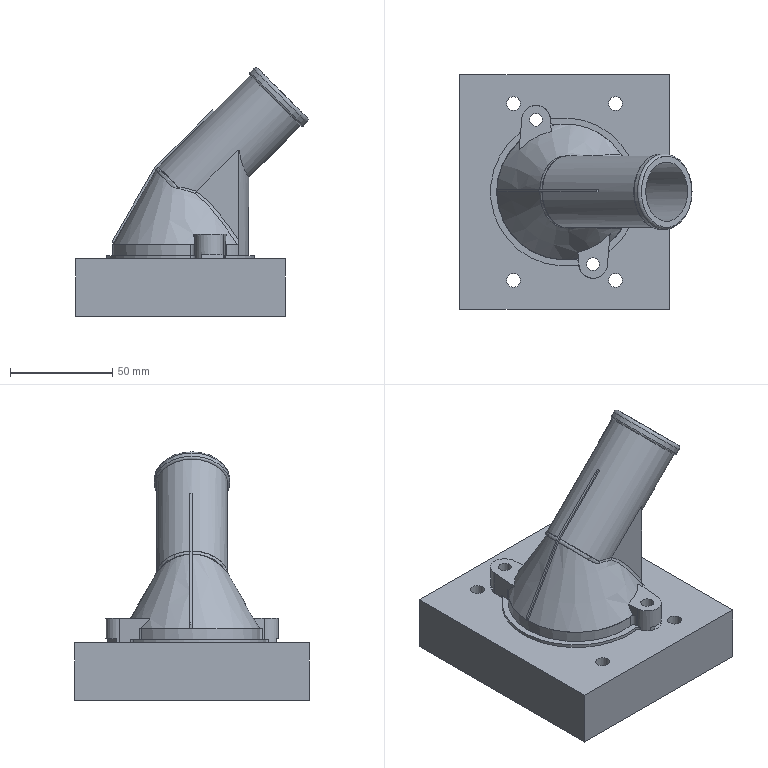NC program | NX | posted by the shop | part box 113.679 x 114.654 x 121.568 mm
Lines 1 to 901 of 160120:
1 BEGIN PGM A MM
2 BLK FORM 0.1 Z X-200 Y-200 Z-20
3 BLK FORM 0.2  X+200  Y+200  Z+0
4 CYCL DEF 247 DATUM SETTING ~
Q339=+1
5 * - OPERATION: 动态开粗 - TOOL: T16 C-D16
6 M5
7 M9
8 PLANE RESET STAY
9 CALL LBL100
10 ;(C-D16 D=16. R=0.)
11 M01
12 TOOL CALL 16 Z S7000
13 CALL LBL101
14 M3 M8
15 M51
16 CYCL DEF 7.0
17 CYCL DEF 7.1 X0
18 CYCL DEF 7.2 Y0
19 CYCL DEF 7.3 Z0
20 CYCL DEF 32.0 TOLERANCE
21 CYCL DEF 32.1 T0.096
22 CYCL DEF 32.2 HSC-MODE:0
23 L M126
24 L A+0.0 C+0.0 FMAX
25 L X-51.5271 Y43.1973 FMAX
26 L Z125.5681 FMAX
27 L Z93.8681 FMAX
28 L Z90.8681 F4000.
29 L X-48.7505 Y43.2945
30 CC X-48.8088 Y44.9119
31 C X-47.2984 Y44.3304 DR+
32 CC X-37.1787 Y41.3645
33 C X-40.3507 Y51.4215 DR-
34 CC X-31.9067 Y24.6985
35 C X-31.7967 Y52.7236 DR-
36 CC X-20.4787 Y-577.0261
37 C X-18.9226 Y52.8234 DR-
38 L X63.2548 Y52.7913
39 CC X62.141 Y43.2465
40 C X70.9126 Y47.1712 DR-
41 CC X51.7584 Y38.5948
42 C X72.7399 Y39.0565 DR-
43 CC X-228.59 Y28.1117
44 C X72.9273 Y25.497 DR-
45 L X72.8975 Y-43.1756
46 CC X63.3192 Y-41.9959
47 C X67.3008 Y-50.7869 DR-
48 CC X58.6418 Y-31.5347
49 C X59.0657 Y-52.6403 DR-
50 CC X47.5617 Y276.8316
51 C X44.3187 Y-52.8251 DR-
52 L X-37.0653 Y-52.7938
53 CC X-35.9739 Y-43.2861
54 C X-44.6673 Y-47.2875 DR-
55 CC X-25.6559 Y-38.5866
56 C X-46.5597 Y-38.9996 DR-
57 CC X275.7523 Y-27.5499
58 C X-46.7468 Y-24.3151 DR-
59 L X-46.7148 Y40.99
60 CC X-35.4927 Y39.7742
61 C X-39.9835 Y50.1301 DR-
62 CC X-30.2581 Y27.4594
63 C X-30.7546 Y52.1231 DR-
64 CC X-18.8584 Y-278.6943
65 C X-15.8203 Y52.323 DR-
66 L X60.7546 Y52.2952
67 CC X59.7468 Y40.9074
68 C X70.2295 Y45.4691 DR-
69 CC X47.4521 Y35.7059
70 C X72.2293 Y36.1782 DR-
71 CC X-271.0461 Y24.0753
72 C X72.427 Y20.8063 DR-
73 L X72.398 Y-40.642
74 CC X60.9905 Y-39.6267
75 C X65.51 Y-50.1498 DR-
76 CC X55.7485 Y-27.1289
77 C X56.2158 Y-52.1295 DR-
78 CC X43.9517 Y302.8918
79 C X40.5313 Y-52.3248 DR-
80 L X-34.5655 Y-52.2948
81 CC X-33.5522 Y-40.8903
82 C X-44.0714 Y-45.4111 DR-
83 CC X-21.1462 Y-35.6768
84 C X-46.0475 Y-36.1746 DR-
85 CC X283.0799 Y-24.3678
86 C X-46.2466 Y-21.4903 DR-
87 L X-46.2165 Y38.7401
88 CC X-33.6191 Y37.9186
89 C X-38.4122 Y49.5974 DR-
90 CC X-28.0851 Y24.1526
91 C X-28.7365 Y51.6055 DR-
92 CC X-16.2771 Y-280.8683
93 C X-12.99 Y51.8227 DR-
94 L X58.6917 Y51.7904
95 CC X57.9108 Y39.0584
96 C X69.7529 Y43.7996 DR-
97 CC X43.3014 Y33.3709
98 C X71.7302 Y33.8628 DR-
99 CC X-257.1344 Y22.4602
100 C X71.9262 Y21.4282 DR-
101 L X71.8928 Y-38.5792
102 CC X59.1566 Y-37.7998
103 C X63.9165 Y-49.6388 DR-
104 CC X53.6366 Y-23.8682
105 C X54.353 Y-51.6043 DR-
106 CC X42.6945 Y245.2934
107 C X40.3567 Y-51.8239 DR-
108 L X-32.627 Y-51.7817
109 CC X-31.7152 Y-39.0403
110 C X-43.5885 Y-43.7519 DR-
111 CC X-17.4661 Y-33.4645
112 C X-45.5335 Y-34.1207 DR-
113 CC X306.6819 Y-21.3815
114 C X-45.7464 Y-17.874 DR-
115 L X-45.7197 Y36.7406
116 CC X-32.0057 Y36.3223
117 C X-36.8804 Y49.1475 DR-
118 CC X-25.9909 Y20.139
119 C X-26.5551 Y51.119 DR-
120 CC X-13.8254 Y-325.6529
121 C X-10.8706 Y51.3224 DR-
122 L X56.7549 Y51.2929
123 CC X56.3438 Y37.4892
124 C X69.2608 Y42.374 DR-
125 CC X40.4784 Y31.582
126 C X71.2093 Y32.2947 DR-
127 CC X-244.4989 Y20.4859
128 C X71.4258 Y18.8606 DR-
129 L X71.3999 Y-36.5391
130 CC X57.5671 Y-36.2198
131 C X62.4086 Y-49.1816 DR-
132 CC X51.6556 Y-20.2511
133 C X52.3894 Y-51.1066 DR-
134 CC X39.7327 Y296.6216
135 C X36.7053 Y-51.3237 DR-
136 L X-30.5651 Y-51.2919
137 CC X-30.1524 Y-37.4747
138 C X-43.102 Y-42.3112 DR-
139 CC X-14.164 Y-31.5543
140 C X-45.0278 Y-32.2923 DR-
141 CC X303.7136 Y-19.5871
142 C X-45.2459 Y-16.5456 DR-
143 L X-45.2191 Y34.9905
144 CC X-30.5699 Y34.8923
145 C X-35.4883 Y48.6915 DR-
146 CC X-24.2496 Y16.9285
147 C X-24.8966 Y50.615 DR-
148 CC X-11.6342 Y-349.5949
149 C X-8.4621 Y50.8221 DR-
150 L X55.1301 Y50.7887
151 CC X54.9378 Y36.0809
152 C X68.7973 Y41.0075 DR-
153 CC X37.3518 Y29.861
154 C X70.7049 Y30.658 DR-
155 CC X-291.953 Y17.6255
156 C X70.9258 Y14.5363 DR-
157 L X70.8911 Y-35.017
158 CC X56.1815 Y-34.8283
159 C X61.1555 Y-48.6728 DR-
160 CC X49.945 Y-17.28
161 C X50.6908 Y-50.606 DR-
162 CC X37.5428 Y324.1744
163 C X34.3815 Y-50.8233 DR-
164 L X-28.8775 Y-50.7902
165 CC X-28.7461 Y-36.0705
166 C X-42.6166 Y-40.9997 DR-
167 CC X-10.2128 Y-29.6263
168 C X-44.5505 Y-30.1571 DR-
169 CC X384.1134 Y-16.8893
170 C X-44.7458 Y-13.9722 DR-
171 L X-44.7146 Y33.4904
172 CC X-29.4154 Y33.634
173 C X-38.3373 Y46.0632 DR-
174 CC X-25.8774 Y27.151
175 C X-28.1768 Y49.6817 DR-
176 CC X-15.9172 Y-66.1755
177 C X-13.888 Y50.3109 DR-
178 L X53.5673 Y50.2877
179 CC X53.6649 Y34.8342
180 C X68.2355 Y39.9837 DR-
181 CC X34.5303 Y28.2436
182 C X70.2157 Y28.8949 DR-
183 CC X-342.2851 Y15.364
184 C X70.4255 Y12.2103 DR-
185 L X70.3935 Y-33.3768
186 CC X54.9211 Y-33.5345
187 C X65.0415 Y-45.2391 DR-
188 CC X52.1569 Y-28.8529
189 C X54.8411 Y-49.5245 DR-
190 CC X42.8171 Y41.5436
191 C X41.2515 Y-50.3015 DR-
192 L X-27.3778 Y-50.2868
193 CC X-27.4802 Y-34.833
194 C X-42.0361 Y-40.0251 DR-
195 CC X-8.7962 Y-28.3311
196 C X-44.0255 Y-29.0629 DR-
197 CC X321.9506 Y-16.1761
198 C X-44.2451 Y-13.8786 DR-
199 L X-44.2075 Y32.1776
200 CC X-27.7349 Y32.303
201 C X-40.0647 Y43.2271 DR-
202 CC X-26.3019 Y29.6858
203 C X-29.7464 Y48.6837 DR-
204 CC X-17.8895 Y-15.9792
205 C X-17.3126 Y49.7592 DR-
206 L X-5.5004 Y49.8213
207 L X52.1921 Y49.7837
208 CC X52.3246 Y33.1488
209 C X63.0764 Y45.8427 DR-
210 CC X50.033 Y31.9896
211 C X68.7144 Y35.6013 DR-
212 CC X7.2893 Y23.6891
213 C X69.8567 Y23.1754 DR-
214 L X69.9251 Y10.4883
215 L X69.897 Y-31.7673
216 CC X52.703 Y-32.0564
217 C X66.7044 Y-42.0403 DR-
218 CC X52.546 Y-30.7301
219 C X56.5272 Y-48.4087 DR-
220 CC X44.7599 Y3.674
221 C X44.6881 Y-49.7214 DR-
222 CC X33.1286 Y594.1964
223 C X31.2513 Y-49.8224 DR-
224 L X-26.0028 Y-49.7828
225 CC X-26.135 Y-33.122
226 C X-36.8355 Y-45.893 DR-
227 CC X-23.9055 Y-32.0177
228 C X-42.5158 Y-35.6737 DR-
229 CC X19.1406 Y-23.6226
230 C X-43.6794 Y-22.9999 DR-
231 L X-43.7452 Y-10.7503
232 L X-43.7128 Y30.6155
233 CC X-25.5099 Y30.8812
234 C X-40.7399 Y40.8542 DR-
235 CC X-26.0631 Y30.0284
236 C X-30.3391 Y47.7576 DR-
237 CC X-18.3723 Y-1.4917
238 C X-18.6416 Y49.1899 DR-
239 CC X-5.5456 Y-598.5509
240 C X-4.2053 Y49.3209 DR-
241 L X50.7546 Y49.285
242 CC X50.9738 Y31.1701
243 C X61.1331 Y46.1697 DR-
244 CC X49.9833 Y31.5306
245 C X67.8898 Y35.7706 DR-
246 CC X18.1827 Y23.873
247 C X69.2928 Y24.1942 DR-
248 CC X-590.6615 Y10.866
249 C X69.4248 Y9.0078 DR-
250 L X69.3879 Y-30.6418
251 CC X51.2087 Y-30.8524
252 C X66.3519 Y-40.9128 DR-
253 CC X51.6791 Y-29.9581
254 C X55.9789 Y-47.7572 DR-
255 CC X43.7101 Y3.3245
256 C X43.6554 Y-49.2099 DR-
257 CC X31.5419 Y595.0316
258 C X29.9687 Y-49.3219 DR-
259 L X-24.6277 Y-49.282
260 CC X-24.8144 Y-31.2417
261 C X-34.9918 Y-46.1382 DR-
262 CC X-23.7252 Y-31.4722
263 C X-41.7454 Y-35.6315 DR-
264 CC X11.2113 Y-23.4019
265 C X-43.1391 Y-23.2999 DR-
266 CC X616.5488 Y-11.2689
267 C X-43.2449 Y-8.9882 DR-
268 L X-43.2153 Y29.1778
269 CC X-23.1618 Y29.5228
270 C X-40.8512 Y38.9751 DR-
271 CC X-25.5189 Y29.6689
272 C X-30.4256 Y46.9202 DR-
273 CC X-17.9847 Y2.9879
274 C X-18.5229 Y48.6446 DR-
275 CC X-4.281 Y-517.0928
276 C X-2.3373 Y48.8205 DR-
277 L X49.5622 Y48.7803
278 CC X49.7655 Y29.4819
279 C X59.7988 Y45.9683 DR-
280 CC X49.3836 Y30.8072
281 C X67.1766 Y35.4703 DR-
282 CC X20.5411 Y23.1978
283 C X68.7614 Y23.7323 DR-
284 CC X-566.2365 Y9.2507
285 C X68.9244 Y7.6091 DR-
286 L X68.8944 Y-29.0796
287 CC X48.7336 Y-29.4536
288 C X66.4967 Y-38.9968 DR-
289 CC X51.1408 Y-29.612
290 C X56.0527 Y-46.9253 DR-
291 CC X43.6294 Y-2.9661
292 C X44.2094 Y-48.6433 DR-
293 CC X30.0587 Y502.7336
294 C X28.1489 Y-48.8216 DR-
295 L X-23.3757 Y-48.7792
296 CC X-23.5805 Y-29.4623
297 C X-33.5538 Y-46.0067 DR-
298 CC X-23.2717 Y-30.8597
299 C X-40.9448 Y-35.6363 DR-
300 CC X4.9606 Y-23.2699
301 C X-42.5785 Y-23.7809 DR-
302 CC X577.7338 Y-9.3246
303 C X-42.7445 Y-7.5952 DR-
304 L X-42.7026 Y28.3028
305 CC X-22.2749 Y28.5305
306 C X-40.084 Y38.5393 DR-
307 CC X-24.4972 Y28.6089
308 C X-29.4957 Y46.4015 DR-
309 CC X-16.81 Y1.0578
310 C X-17.4046 Y48.1388 DR-
311 CC X-2.925 Y-515.6188
312 C X-.6567 Y48.3202 DR-
313 L X48.1299 Y48.2853
314 CC X48.4503 Y27.1546
315 C X58.1287 Y45.9412 DR-
316 CC X48.8475 Y30.1525
317 C X66.448 Y35.2168 DR-
318 CC X21.9439 Y22.457
319 C X68.237 Y23.0719 DR-
320 CC X-482.9193 Y8.4598
321 C X68.424 Y5.7616 DR-
322 L X68.3863 Y-28.0755
323 CC X47.3939 Y-28.3732
324 C X65.9882 Y-38.121 DR-
325 CC X50.2289 Y-28.7098
326 C X55.2871 Y-46.3547 DR-
327 CC X42.4454 Y-1.228
328 C X42.9523 Y-48.1435 DR-
329 CC X28.5587 Y524.8483
330 C X26.6418 Y-48.3211 DR-
331 L X-21.9399 Y-48.2844
332 CC X-22.2526 Y-27.0592
333 C X-31.8286 Y-46.0041 DR-
334 CC X-22.7037 Y-30.1758
335 C X-40.2534 Y-35.2557 DR-
336 CC X3.6049 Y-22.567
337 C X-42.0462 Y-23.2998 DR-
338 CC X474.4267 Y-8.6811
339 C X-42.2443 Y-5.6773 DR-
340 L X-42.2054 Y26.9906
341 CC X-20.1128 Y27.2936
342 C X-39.9239 Y37.0759 DR-
343 CC X-23.8274 Y28.0134
344 C X-29.2291 Y45.6783 DR-
345 CC X-16.2757 Y3.0803
346 C X-17.1682 Y47.5952 DR-
347 CC X-2.7231 Y-397.7243
348 C X.2038 Y47.8198 DR-
349 L X47.005 Y47.7821
350 CC X47.3186 Y25.4234
351 C X56.9872 Y45.5859 DR-
352 CC X48.1506 Y29.4233
353 C X65.736 Y34.907 DR-
354 CC X24.2956 Y22.0252
355 C X67.6787 Y23.1011 DR-
356 CC X-368.99 Y7.9553
357 C X67.9237 Y4.0421 DR-
358 L X67.8831 Y-26.9549
359 CC X45.6791 Y-27.2437
360 C X65.6345 Y-36.9844 DR-
361 CC X49.4464 Y-27.9634
362 C X54.7559 Y-45.7185 DR-
363 CC X41.7553 Y-2.1074
364 C X42.5648 Y-47.6078 DR-
365 CC X27.9232 Y433.1742
366 C X24.8176 Y-47.8207 DR-
367 L X-20.8321 Y-47.7808
368 CC X-21.1499 Y-25.5242
369 C X-30.9223 Y-45.5232 DR-
370 CC X-21.8627 Y-29.3237
371 C X-39.6558 Y-34.6061 DR-
372 CC X3.7649 Y-21.7037
373 C X-41.5234 Y-22.6002 DR-
374 CC X412.3699 Y-8.1863
375 C X-41.7438 Y-5.4156 DR-
376 L X-41.7121 Y25.5529
377 CC X-17.3676 Y25.9948
378 C X-39.792 Y35.4814 DR-
379 CC X-23.1265 Y27.3614
380 C X-28.8246 Y45.0024 DR-
381 CC X-15.4686 Y3.2404
382 C X-16.4163 Y47.0759 DR-
383 CC X-2.0076 Y-363.256
384 C X.7678 Y47.3194 DR-
385 L X45.6298 Y47.2872
386 CC X46.0628 Y22.9015
387 C X55.5594 Y45.3662 DR-
388 CC X47.4489 Y28.6837
389 C X65.0933 Y34.4074 DR-
390 CC X23.5706 Y21.0615
391 C X67.1739 Y22.0618 DR-
392 CC X-358.4176 Y7.0624
393 C X67.4233 Y3.5029 DR-
394 L X67.3832 Y-25.7718
395 CC X43.7081 Y-26.094
396 C X65.3096 Y-35.7887 DR-
397 CC X48.7199 Y-27.2622
398 C X54.3924 Y-45.0314 DR-
399 CC X41.1 Y-3.0581
400 C X42.104 Y-47.0744 DR-
401 CC X27.5018 Y367.286
402 C X24.4201 Y-47.3202 DR-
403 L X-19.4407 Y-47.2863
404 CC X-19.8747 Y-22.8673
405 C X-29.3691 Y-45.3692 DR-
406 CC X-21.2838 Y-28.7022
407 C X-38.8817 Y-34.4877 DR-
408 CC X2.1771 Y-21.1275
409 C X-40.9886 Y-22.1485 DR-
410 CC X374.983 Y-7.1518
411 C X-41.2436 Y-3.5897 DR-
412 L X-41.2012 Y24.8027
413 CC X-16.5669 Y25.1038
414 C X-39.1965 Y34.8426 DR-
415 CC X-22.2351 Y26.4689
416 C X-27.951 Y44.5004 DR-
417 CC X-14.4415 Y1.6581
418 C X-15.4752 Y46.568 DR-
419 CC X-.5732 Y-374.1738
420 C X2.7087 Y46.819 DR-
421 L X44.5459 Y46.7853
422 CC X44.9837 Y21.1151
423 C X54.5569 Y44.9375 DR-
424 CC X46.6875 Y27.9166
425 C X64.4563 Y33.9091 DR-
426 CC X24.6152 Y20.5328
427 C X66.6176 Y21.958 DR-
428 CC X-287.3896 Y6.8106
429 C X66.9227 Y3.1507 DR-
430 L X66.8811 Y-24.7048
431 CC X42.1762 Y-25.0478
432 C X64.8259 Y-34.919 DR-
433 CC X47.8826 Y-26.4324
434 C X53.6463 Y-44.4845 DR-
435 CC X40.0592 Y-1.5573
436 C X41.05 Y-46.5726 DR-
437 CC X25.9861 Y388.1239
438 C X22.5535 Y-46.82 DR-
439 L X-18.253 Y-46.7871
440 CC X-18.7299 Y-20.6873
441 C X-28.2162 Y-45.0068 DR-
442 CC X-20.4745 Y-27.8745
443 C X-38.3406 Y-33.7271 DR-
444 CC X3.5275 Y-20.1264
445 C X-40.4812 Y-21.2012 DR-
446 CC X386.1096 Y-5.7405
447 C X-40.7433 Y-1.8301 DR-
448 L X-40.705 Y23.553
449 CC X-14.3291 Y23.9535
450 C X-38.8447 Y33.6919 DR-
451 CC X-21.5275 Y25.7712
452 C X-27.5683 Y43.8303 DR-
453 CC X-13.8701 Y2.5862
454 C X-15.1787 Y46.0259 DR-
455 CC X.4776 Y-344.5899
456 C X4.5041 Y46.3187 DR-
457 L X43.63 Y46.2802
458 CC X44.0252 Y19.862
459 C X53.7682 Y44.4211 DR-
460 CC X45.8509 Y27.0759
461 C X63.9413 Y33.099 DR-
462 CC X22.4223 Y19.3688
463 C X66.134 Y20.6461 DR-
464 CC X-325.094 Y5.1321
465 C X66.4225 Y1.2757 DR-
466 L X66.375 Y-23.8114
467 CC X40.9467 Y-24.0965
468 C X64.3272 Y-34.0983 DR-
469 CC X47.1149 Y-25.6642
470 C X53.1288 Y-43.8638 DR-
471 CC X39.445 Y-2.1483
472 C X40.7361 Y-46.0319 DR-
473 CC X25.5634 Y332.681
474 C X22.0532 Y-46.3194 DR-
475 L X-17.4406 Y-46.2795
476 CC X-17.8279 Y-19.7455
477 C X-27.5215 Y-44.4485 DR-
478 CC X-19.6709 Y-27.0766
479 C X-37.7501 Y-33.1229 DR-
480 CC X3.5864 Y-19.3933
481 C X-39.9517 Y-20.6744 DR-
482 CC X349.2838 Y-5.1237
483 C X-40.2429 Y-1.2415 DR-
484 L X-40.2028 Y22.5528
485 CC X-12.7104 Y22.9506
486 C X-38.3925 Y32.7698 DR-
487 CC X-20.7046 Y24.9568
488 C X-26.7651 Y43.3192 DR-
489 CC X-13.0092 Y1.6482
490 C X-14.4993 Y45.5056 DR-
491 CC X1.1984 Y-323.7353
492 C X5.1204 Y45.8184 DR-
493 L X42.2702 Y45.7867
494 CC X42.7922 Y16.8331
495 C X52.3961 Y44.1525 DR-
496 CC X45.1567 Y26.3709
497 C X63.3027 Y32.6411 DR-
498 CC X22.6619 Y18.7004
499 C X65.6029 Y20.1471 DR-
500 CC X-294.081 Y4.5082
501 C X65.9221 Y.6526 DR-
502 L X65.8761 Y-22.7044
503 CC X39.0132 Y-23.0309
504 C X63.9514 Y-33.0212 DR-
505 CC X46.317 Y-24.8842
506 C X52.3472 Y-43.3455 DR-
507 CC X38.3494 Y-.1781
508 C X39.5178 Y-45.5433 DR-
509 CC X23.9356 Y368.3583
510 C X20.147 Y-45.8192 DR-
511 L X-16.0654 Y-45.7864
512 CC X-16.598 Y-16.7638
513 C X-26.1922 Y-44.1599 DR-
514 CC X-18.9456 Y-26.3345
515 C X-37.1697 Y-32.5103 DR-
516 CC X4.0707 Y-18.5957
517 C X-39.431 Y-20.0083 DR-
518 CC X305.5622 Y-5.0345
519 C X-39.742 Y-1.951 DR-
520 L X-39.6964 Y21.74
521 CC X-11.8339 Y22.0825
522 C X-37.8009 Y32.1896 DR-
523 CC X-19.9345 Y24.1779
524 C X-26.1681 Y42.7396 DR-
525 CC X-11.982 Y.1115
526 C X-13.2889 Y45.0191 DR-
527 CC X2.1441 Y-332.9092
528 C X5.6438 Y45.3179 DR-
529 L X41.1922 Y45.287
530 CC X41.7257 Y14.5314
531 C X51.2799 Y43.7702 DR-
532 CC X44.4396 Y25.6579
533 C X62.6649 Y32.1912 DR-
534 CC X22.5128 Y17.9669
535 C X65.0834 Y19.4706 DR-
536 CC X-299.1991 Y3.1824
537 C X65.4217 Y-1.1484 DR-
538 CC X-725.83 Y-8.4369
539 C X65.318 Y-23.1719 DR-
540 CC X41.4457 Y-22.8814
541 C X62.6126 Y-33.9237 DR-
542 CC X45.2211 Y-23.6971
543 C X51.0572 Y-43.01 DR-
544 CC X37.1856 Y2.8375
545 C X38.5064 Y-45.0443 DR-
546 CC X22.9936 Y370.4271
547 C X19.448 Y-45.3187 DR-
548 L X-15.0026 Y-45.2864
549 CC X-15.5709 Y-14.8499
550 C X-25.2677 Y-43.706 DR-
551 CC X-18.1895 Y-25.5791
552 C X-36.5871 Y-31.9205 DR-
553 CC X4.0418 Y-17.9365
554 C X-38.8935 Y-19.6158 DR-
555 CC X319.2903 Y-3.1942
556 C X-39.2421 Y1.2529 DR-
557 CC X650.7968 Y8.181
558 C X-39.1298 Y22.4266 DR-
559 CC X-14.8636 Y22.068
560 C X-36.4079 Y33.2403 DR-
561 CC X-18.8024 Y22.9555
562 C X-24.714 Y42.4692 DR-
563 CC X-10.5568 Y-4.3171
564 C X-11.7948 Y44.5486 DR-
565 CC X3.9565 Y-391.2903
566 C X7.6388 Y44.8176 DR-
567 L X40.3176 Y44.7835
568 CC X40.8607 Y13.7191
569 C X50.7649 Y43.1673 DR-
570 CC X43.6262 Y24.8453
571 C X62.1642 Y31.4028 DR-
572 CC X21.4403 Y17.11
573 C X64.5687 Y18.7409 DR-
574 CC X-291.149 Y2.321
575 C X64.9212 Y-2.0027 DR-
576 CC X-592.9356 Y-8.5542
577 C X64.8084 Y-22.3907 DR-
578 CC X40.5507 Y-22.0424
579 C X62.0333 Y-33.3141 DR-
580 CC X44.4908 Y-22.9618
581 C X50.549 Y-42.4095 DR-
582 CC X36.4391 Y3.0518
583 C X37.8275 Y-44.5285 DR-
584 CC X21.6549 Y377.0228
585 C X17.5194 Y-44.8183 DR-
586 L X-14.1282 Y-44.783
587 CC X-14.6417 Y-13.3478
588 C X-24.4002 Y-43.2344 DR-
589 CC X-17.4302 Y-24.8201
590 C X-36.0307 Y-31.2767 DR-
591 CC X5.5255 Y-16.9457
592 C X-38.4056 Y-18.4783 DR-
593 CC X331.2991 Y-2.1523
594 C X-38.7417 Y2.0783 DR-
595 CC X575.1287 Y8.1712
596 C X-38.6261 Y21.5513 DR-
597 CC X-13.8076 Y21.1972
598 C X-35.8786 Y32.553 DR-
599 CC X-18.101 Y22.2551
600 C X-24.2562 Y41.8562 DR-
601 CC X-9.8296 Y-4.4477
602 C X-11.1007 Y44.0349 DR-
603 CC X5.2482 Y-397.7274
604 C X9.4576 Y44.3173 DR-
605 L X39.6925 Y44.2745
606 CC X40.0945 Y13.1656
607 C X50.1332 Y42.613 DR-
608 CC X42.836 Y24.0537
609 C X61.6663 Y30.62 DR-
610 CC X20.1141 Y16.2044
611 C X64.0635 Y17.8908 DR-
612 CC X-285.5371 Y1.5589
613 C X64.4208 Y-2.5402 DR-
614 CC X-451.6653 Y-8.6286
615 C X64.2882 Y-21.813 DR-
616 CC X40.0834 Y-21.3265
617 C X61.3258 Y-32.9399 DR-
618 CC X43.6225 Y-22.0661
619 C X49.5961 Y-41.9649 DR-
620 CC X35.3149 Y5.6521
621 C X36.6106 Y-44.0435 DR-
622 CC X21.1953 Y372.0183
623 C X18.1146 Y-44.3176 DR-
624 L X-13.2528 Y-44.2799
625 CC X-13.7659 Y-12.2879
626 C X-23.7689 Y-42.6802 DR-
627 CC X-16.6975 Y-24.0989
628 C X-35.4184 Y-30.7919 DR-
629 CC X5.5759 Y-16.2797
630 C X-37.8792 Y-17.9504 DR-
631 CC X310.1243 Y-1.5395
632 C X-38.2413 Y2.6055 DR-
633 CC X416.1291 Y8.3503
634 C X-38.0979 Y21.128 DR-
635 CC X-13.7078 Y20.5794
636 C X-35.0401 Y32.4164 DR-
637 CC X-17.2378 Y21.3487
638 C X-23.3876 Y41.3885 DR-
639 CC X-8.8619 Y-6.2775
640 C X-10.165 Y43.5356 DR-
641 CC X5.5673 Y-376.8968
642 C X8.8933 Y43.8167 DR-
643 L X38.4427 Y43.7806
644 CC X38.9569 Y10.1262
645 C X48.9148 Y42.2778 DR-
646 CC X42.1424 Y23.3595
647 C X61.0686 Y30.1096 DR-
648 CC X20.2503 Y15.6061
649 C X63.5265 Y17.5203 DR-
650 CC X-287.3435 Y.1917
651 C X63.9206 Y-4.6595 DR-
652 CC X-258.5757 Y-9.7285
653 C X63.7405 Y-21.639 DR-
654 CC X40.395 Y-20.8408
655 C X60.2371 Y-33.1671 DR-
656 CC X42.5932 Y-20.9281
657 C X48.3575 Y-41.6132 DR-
658 CC X33.8138 Y10.7222
659 C X34.7864 Y-43.5877 DR-
660 CC X19.1467 Y470.1523
661 C X16.2267 Y-43.8174 DR-
662 L X-12.298 Y-43.7793
663 CC X-12.8173 Y-10.5238
664 C X-22.8859 Y-42.2227 DR-
665 CC X-15.9713 Y-23.3732
666 C X-34.8575 Y-30.1866 DR-
667 CC X6.0756 Y-15.551
668 C X-37.3581 Y-17.3502 DR-
669 CC X319.7513 Y-.1329
670 C X-37.741 Y4.6425 DR-
671 CC X262.6443 Y9.3394
672 C X-37.5567 Y20.8618 DR-
673 CC X-13.6968 Y20.0266
674 C X-34.1719 Y32.3052 DR-
675 CC X-16.3205 Y20.3701
676 C X-22.3197 Y40.9888 DR-
677 CC X-7.7115 Y-9.3315
678 C X-8.9525 Y43.0516 DR-
679 CC X7.1726 Y-422.6598
680 C X10.7938 Y43.3166 DR-
681 L X37.5673 Y43.2786
682 CC X38.0993 Y9.0234
683 C X48.2843 Y41.7338 DR-
684 CC X41.3799 Y22.5936
685 C X60.5746 Y29.3451 DR-
686 CC X18.5847 Y14.641
687 C X63.0358 Y16.5007 DR-
688 CC X-290.3909 Y-.6078
689 C X63.4201 Y-5.1796 DR-
690 CC X-216.4956 Y-9.7345
691 C X63.2399 Y-20.7635 DR-
692 CC X39.2148 Y-19.964
693 C X59.8945 Y-32.2194 DR-
694 CC X41.9902 Y-20.3722
695 C X47.9895 Y-40.986 DR-
696 CC X33.4888 Y8.7437
697 C X34.8742 Y-43.0385 DR-
698 CC X18.3077 Y417.9391
699 C X14.1282 Y-43.3171 DR-
700 L X-11.253 Y-43.2809
701 CC X-11.7985 Y-8.0452
702 C X-21.8001 Y-41.8361 DR-
703 CC X-15.214 Y-22.6026
704 C X-34.3939 Y-29.343 DR-
705 CC X8.0295 Y-14.5301
706 C X-36.8728 Y-16.249 DR-
707 CC X329.0858 Y.7632
708 C X-37.2406 Y5.2443 DR-
709 CC X197.9024 Y9.4555
710 C X-37.0195 Y20.4855 DR-
711 CC X-13.5209 Y19.4418
712 C X-33.2692 Y32.2198 DR-
713 CC X-15.4342 Y19.4069
714 C X-21.377 Y40.5479 DR-
715 CC X-6.6427 Y-11.9531
716 C X-7.8113 Y42.5637 DR-
717 CC X8.2431 Y-445.2317
718 C X11.6228 Y42.8162 DR-
719 L X36.8975 Y42.7724
720 CC X37.3063 Y7.9993
721 C X47.4946 Y41.2488 DR-
722 CC X40.6958 Y21.9199
723 C X59.9618 Y28.8951 DR-
724 CC X18.2886 Y13.9454
725 C X62.5224 Y15.8201 DR-
726 CC X-288.1204 Y-1.5006
727 C X62.9197 Y-6.1097 DR-
728 CC X-136.64 Y-10.0979
729 C X62.6779 Y-20.6989 DR-
730 CC X39.5834 Y-19.5446
731 C X58.6498 Y-32.6274 DR-
732 CC X40.9876 Y-19.2168
733 C X46.9279 Y-40.5829 DR-
734 CC X32.378 Y11.7379
735 C X33.7325 Y-42.5514 DR-
736 CC X17.9302 Y410.6868
737 C X14.8611 Y-42.8164 DR-
738 L X-10.5386 Y-42.7759
739 CC X-11.0236 Y-7.3512
740 C X-21.2041 Y-41.285 DR-
741 CC X-14.524 Y-21.9281
742 C X-33.7652 Y-28.9346 DR-
743 CC X7.3986 Y-14.0573
744 C X-36.3258 Y-16.0482 DR-
745 CC X304.0923 Y1.3921
746 C X-36.7402 Y6.0685 DR-
747 CC X148.4404 Y9.6867
748 C X-36.4856 Y20.0465 DR-
749 CC X-13.1255 Y18.8137
750 C X-32.4883 Y31.9399 DR-
751 CC X-14.5731 Y18.4811
752 C X-20.4259 Y40.1106 DR-
753 CC X-5.5014 Y-15.1248
754 C X-6.538 Y42.082 DR-
755 CC X9.9178 Y-508.8564
756 C X13.5216 Y42.3159 DR-
757 CC X21.5805 Y-891.3128
758 C X37.8788 Y42.2084 DR-
759 CC X37.6304 Y13.711
760 C X48.9921 Y39.8468 DR-
761 CC X39.6796 Y20.9386
762 C X59.6771 Y27.5975 DR-
763 CC X14.6395 Y12.6516
764 C X62.0593 Y14.4182 DR-
765 CC X-360.3702 Y-3.8649
766 C X62.4196 Y-9.3255 DR-
767 CC X-39.5118 Y-11.9286
768 C X61.9969 Y-21.56 DR-
769 CC X40.8432 Y-19.5538
770 C X55.4085 Y-35.0249 DR-
771 CC X38.6623 Y-15.6077
772 C X43.4178 Y-40.8039 DR-
773 CC X28.6512 Y36.6567
774 C X28.8188 Y-42.1987 DR-
775 CC X15.5664 Y659.2429
776 C X12.3197 Y-42.3164 DR-
777 CC X4.4682 Y879.8962
778 C X-11.6893 Y-42.2082 DR-
779 CC X-11.4243 Y-13.5549
780 C X-22.688 Y-39.9028 DR-
781 CC X-13.5278 Y-20.9601
782 C X-33.4807 Y-27.6396 DR-
783 CC X10.9911 Y-12.7661
784 C X-35.8643 Y-14.648 DR-
785 CC X375.3576 Y3.7937
786 C X-36.2401 Y9.3452 DR-
787 CC X49.7973 Y11.7321
788 C X-35.7089 Y21.5723 DR-
789 CC X-14.8311 Y19.0498
790 C X-21.8228 Y38.8831 DR-
791 CC X-6.7285 Y-4.1878
792 C X-8.7341 Y41.4074 DR-
793 CC X9.3893 Y-328.5944
794 C X14.508 Y41.8156 DR-
795 CC X21.729 Y-775.1165
796 C X37.1564 Y41.7018 DR-
797 CC X36.8698 Y12.893
798 C X48.3869 Y39.3011 DR-
799 CC X39.0156 Y20.2819
800 C X59.0745 Y27.1515 DR-
801 CC X15.2819 Y12.1902
802 C X61.5144 Y14.238 DR-
803 CC X-284.3844 Y-3.0593
804 C X61.9188 Y-7.4418 DR-
805 CC X-60.3268 Y-10.3774
806 C X61.5454 Y-20.367 DR-
807 CC X39.5003 Y-18.5749
808 C X56.0683 Y-33.2275 DR-
809 CC X38.7515 Y-16.4404
810 C X44.1756 Y-39.9405 DR-
811 CC X29.2967 Y24.4146
812 C X30.0545 Y-41.6338 DR-
813 CC X14.3482 Y631.9529
814 C X13.0563 Y-41.8156 DR-
815 CC X5.1546 Y880.9524
816 C X-10.7175 Y-41.713 DR-
817 CC X-10.5197 Y-12.0478
818 C X-21.8574 Y-39.4616 DR-
819 CC X-12.8934 Y-20.3282
820 C X-32.8557 Y-27.2529 DR-
821 CC X11.5331 Y-12.013
822 C X-35.3655 Y-13.7845 DR-
823 CC X372.0777 Y4.45
824 C X-35.5738 Y17.2058 DR-
825 CC X-8.5143 Y16.4987
826 C X-32.7658 Y28.5229 DR-
827 CC X-13.8556 Y18.0197
828 C X-20.5838 Y38.578 DR-
829 CC X-5.2682 Y-8.634
830 C X-6.8997 Y40.9733 DR-
831 CC X9.8766 Y-348.4503
832 C X13.7822 Y41.3149 DR-
833 CC X21.0134 Y-736.6575
834 C X36.441 Y41.1955 DR-
835 CC X36.1121 Y12.0373
836 C X47.7342 Y38.7812 DR-
837 CC X38.3078 Y19.571
838 C X58.5696 Y26.4518 DR-
839 CC X13.9399 Y11.3299
840 C X61.0187 Y13.3493 DR-
841 CC X-320.127 Y-4.8736
842 C X61.4159 Y-10.2681 DR-
843 CC X-5.9038 Y-11.9867
844 C X60.7289 Y-21.7325 DR-
845 CC X39.8296 Y-18.3865
846 C X46.8882 Y-38.3402 DR-
847 CC X31.5009 Y5.5536
848 C X33.3698 Y-40.9216 DR-
849 CC X15.8625 Y321.8132
850 C X11.3146 Y-41.3154 DR-
851 CC X4.3559 Y591.3903
852 C X-10.6262 Y-41.1763 DR-
853 CC X-10.1431 Y-13.0154
854 C X-21.9936 Y-38.566 DR-
855 CC X-12.0449 Y-19.5068
856 C X-32.4244 Y-26.3556 DR-
857 CC X13.1331 Y-11.1373
858 C X-34.8632 Y-12.9904 DR-
859 CC X332.4628 Y4.2669
860 C X-35.0627 Y16.5622 DR-
861 CC X-7.9671 Y15.8125
862 C X-32.1263 Y28.1034 DR-
863 CC X-13.1577 Y17.3082
864 C X-19.9959 Y38.0346 DR-
865 CC X-4.7358 Y-8.4529
866 C X-6.6303 Y40.4385 DR-
867 CC X10.3595 Y-322.6141
868 C X14.3005 Y40.8145 DR-
869 CC X21.2179 Y-557.7913
870 C X36.1357 Y40.6685 DR-
871 CC X35.596 Y12.2501
872 C X47.5635 Y38.0315 DR-
873 CC X37.4972 Y18.7782
874 C X58.1402 Y25.5521 DR-
875 CC X11.3309 Y10.2293
876 C X60.5502 Y12.0608 DR-
877 CC X-277.4362 Y-4.4041
878 C X60.7238 Y-16.804 DR-
879 CC X34.1818 Y-15.9348
880 C X57.6166 Y-28.4265 DR-
881 CC X38.7322 Y-17.1855
882 C X45.457 Y-38.1082 DR-
883 CC X30.2855 Y9.1896
884 C X32.2021 Y-40.4449 DR-
885 CC X14.1403 Y366.0553
886 C X9.146 Y-40.8153 DR-
887 CC X3.2839 Y406.2301
888 C X-10.3135 Y-40.6469 DR-
889 CC X-9.6329 Y-13.1964
890 C X-21.867 Y-37.7793 DR-
891 CC X-11.2358 Y-18.7245
892 C X-31.9636 Y-25.5411 DR-
893 CC X15.1465 Y-10.1614
894 C X-34.3793 Y-11.922 DR-
895 CC X306.9353 Y4.1782
896 C X-34.5626 Y15.7562 DR-
897 CC X-6.7687 Y14.9939
898 C X-31.7503 Y27.2005 DR-
899 CC X-12.5194 Y16.6885
900 C X-19.4172 Y37.4911 DR-